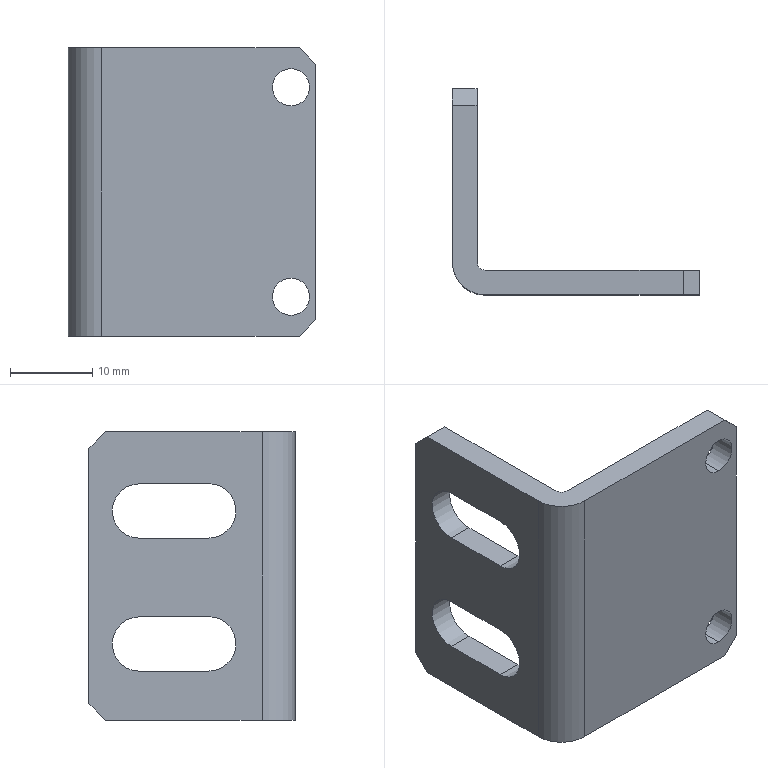Part | SolidWorks | features ICE 3, Chamfer 2, DelFace 2, HoleWzd 2, MoveFace 2, BaseBody 1 | 1 solid | 28 faces | box 30 x 25 x 35 mm | volume 4690 mm3 | plane 16 | cylinder 12 | commonest cylinder face diameters 6.6 x6 4.5 x4 2 x1 8 x1
STEP:
#1=CARTESIAN_POINT('',(-7.,3.,2.55));
#2=VERTEX_POINT('',#1);
#3=CARTESIAN_POINT('',(-7.,3.,7.05));
#4=VERTEX_POINT('',#3);
#5=CARTESIAN_POINT('',(-7.,3.,4.8));
#6=DIRECTION('',(0.,1.,0.));
#7=DIRECTION('',(0.,0.,1.));
#8=AXIS2_PLACEMENT_3D('',#5,#6,#7);
#9=CIRCLE('',#8,2.25);
#10=EDGE_CURVE('',#2,#4,#9,.T.);
#11=ORIENTED_EDGE('',*,*,#10,.T.);
#12=CARTESIAN_POINT('',(-7.,0.,7.05));
#13=VERTEX_POINT('',#12);
#14=CARTESIAN_POINT('',(-7.,0.,7.05));
#15=DIRECTION('',(0.,-1.,0.));
#16=VECTOR('',#15,1000.);
#17=LINE('',#14,#16);
#18=EDGE_CURVE('',#4,#13,#17,.T.);
#19=ORIENTED_EDGE('',*,*,#18,.T.);
#20=CARTESIAN_POINT('',(-7.,0.,2.55));
#21=VERTEX_POINT('',#20);
#22=CARTESIAN_POINT('',(-7.,0.,4.8));
#23=DIRECTION('',(0.,-1.,0.));
#24=DIRECTION('',(0.,0.,-1.));
#25=AXIS2_PLACEMENT_3D('',#22,#23,#24);
#26=CIRCLE('',#25,2.25);
#27=EDGE_CURVE('',#13,#21,#26,.T.);
#28=ORIENTED_EDGE('',*,*,#27,.T.);
#29=CARTESIAN_POINT('',(-7.,0.,2.55));
#30=DIRECTION('',(0.,-1.,0.));
#31=VECTOR('',#30,1000.);
#32=LINE('',#29,#31);
#33=EDGE_CURVE('',#2,#21,#32,.T.);
#34=ORIENTED_EDGE('',*,*,#33,.F.);
#35=EDGE_LOOP('',(#11,#19,#28,#34));
#36=FACE_OUTER_BOUND('',#35,.T.);
#37=CARTESIAN_POINT('',(-7.,0.,4.8));
#38=DIRECTION('',(0.,-1.,0.));
#39=DIRECTION('',(0.,0.,-1.));
#40=AXIS2_PLACEMENT_3D('',#37,#38,#39);
#41=CYLINDRICAL_SURFACE('',#40,2.25);
#42=ADVANCED_FACE('',(#36),#41,.F.);
#43=CARTESIAN_POINT('',(-7.,3.,27.95));
#44=VERTEX_POINT('',#43);
#45=CARTESIAN_POINT('',(-7.,3.,32.45));
#46=VERTEX_POINT('',#45);
#47=CARTESIAN_POINT('',(-7.,3.,30.2));
#48=DIRECTION('',(0.,1.,0.));
#49=DIRECTION('',(0.,0.,1.));
#50=AXIS2_PLACEMENT_3D('',#47,#48,#49);
#51=CIRCLE('',#50,2.25);
#52=EDGE_CURVE('',#44,#46,#51,.T.);
#53=ORIENTED_EDGE('',*,*,#52,.T.);
#54=CARTESIAN_POINT('',(-7.,0.,32.45));
#55=VERTEX_POINT('',#54);
#56=CARTESIAN_POINT('',(-7.,0.,32.45));
#57=DIRECTION('',(0.,-1.,0.));
#58=VECTOR('',#57,1000.);
#59=LINE('',#56,#58);
#60=EDGE_CURVE('',#46,#55,#59,.T.);
#61=ORIENTED_EDGE('',*,*,#60,.T.);
#62=CARTESIAN_POINT('',(-7.,0.,27.95));
#63=VERTEX_POINT('',#62);
#64=CARTESIAN_POINT('',(-7.,0.,30.2));
#65=DIRECTION('',(0.,-1.,0.));
#66=DIRECTION('',(0.,0.,-1.));
#67=AXIS2_PLACEMENT_3D('',#64,#65,#66);
#68=CIRCLE('',#67,2.25);
#69=EDGE_CURVE('',#55,#63,#68,.T.);
#70=ORIENTED_EDGE('',*,*,#69,.T.);
#71=CARTESIAN_POINT('',(-7.,0.,27.95));
#72=DIRECTION('',(0.,-1.,0.));
#73=VECTOR('',#72,1000.);
#74=LINE('',#71,#73);
#75=EDGE_CURVE('',#44,#63,#74,.T.);
#76=ORIENTED_EDGE('',*,*,#75,.F.);
#77=EDGE_LOOP('',(#53,#61,#70,#76));
#78=FACE_OUTER_BOUND('',#77,.T.);
#79=CARTESIAN_POINT('',(-7.,0.,30.2));
#80=DIRECTION('',(0.,-1.,0.));
#81=DIRECTION('',(0.,0.,-1.));
#82=AXIS2_PLACEMENT_3D('',#79,#80,#81);
#83=CYLINDRICAL_SURFACE('',#82,2.25);
#84=ADVANCED_FACE('',(#78),#83,.F.);
#85=CARTESIAN_POINT('',(-31.,10.466,12.573));
#86=VERTEX_POINT('',#85);
#87=CARTESIAN_POINT('',(-31.,10.476,12.573));
#88=VERTEX_POINT('',#87);
#89=CARTESIAN_POINT('',(-31.,10.466,9.273));
#90=DIRECTION('',(-1.,0.,0.));
#91=DIRECTION('',(0.,0.,1.));
#92=AXIS2_PLACEMENT_3D('',#89,#90,#91);
#93=CIRCLE('',#92,3.3);
#94=EDGE_CURVE('',#86,#88,#93,.T.);
#95=ORIENTED_EDGE('',*,*,#94,.F.);
#96=CARTESIAN_POINT('',(-34.,10.466,12.573));
#97=VERTEX_POINT('',#96);
#98=CARTESIAN_POINT('',(-34.,10.466,12.573));
#99=DIRECTION('',(-1.,0.,0.));
#100=VECTOR('',#99,1000.);
#101=LINE('',#98,#100);
#102=EDGE_CURVE('',#86,#97,#101,.T.);
#103=ORIENTED_EDGE('',*,*,#102,.T.);
#104=CARTESIAN_POINT('',(-34.,10.476,12.573));
#105=VERTEX_POINT('',#104);
#106=CARTESIAN_POINT('',(-34.,10.466,9.273));
#107=DIRECTION('',(-1.,0.,0.));
#108=DIRECTION('',(0.,0.,1.));
#109=AXIS2_PLACEMENT_3D('',#106,#107,#108);
#110=CIRCLE('',#109,3.3);
#111=EDGE_CURVE('',#97,#105,#110,.T.);
#112=ORIENTED_EDGE('',*,*,#111,.T.);
#113=CARTESIAN_POINT('',(-34.,10.476,12.573));
#114=DIRECTION('',(-1.,0.,0.));
#115=VECTOR('',#114,1000.);
#116=LINE('',#113,#115);
#117=EDGE_CURVE('',#88,#105,#116,.T.);
#118=ORIENTED_EDGE('',*,*,#117,.F.);
#119=EDGE_LOOP('',(#95,#103,#112,#118));
#120=FACE_OUTER_BOUND('',#119,.T.);
#121=CARTESIAN_POINT('',(-34.,10.466,9.273));
#122=DIRECTION('',(-1.,0.,0.));
#123=DIRECTION('',(0.,0.,1.));
#124=AXIS2_PLACEMENT_3D('',#121,#122,#123);
#125=CYLINDRICAL_SURFACE('',#124,3.3);
#126=ADVANCED_FACE('',(#120),#125,.F.);
#127=CARTESIAN_POINT('',(-31.,10.466,28.701));
#128=VERTEX_POINT('',#127);
#129=CARTESIAN_POINT('',(-31.,10.476,28.701));
#130=VERTEX_POINT('',#129);
#131=CARTESIAN_POINT('',(-31.,10.466,25.401));
#132=DIRECTION('',(-1.,0.,0.));
#133=DIRECTION('',(0.,0.,1.));
#134=AXIS2_PLACEMENT_3D('',#131,#132,#133);
#135=CIRCLE('',#134,3.3);
#136=EDGE_CURVE('',#128,#130,#135,.T.);
#137=ORIENTED_EDGE('',*,*,#136,.F.);
#138=CARTESIAN_POINT('',(-34.,10.466,28.701));
#139=VERTEX_POINT('',#138);
#140=CARTESIAN_POINT('',(-34.,10.466,28.701));
#141=DIRECTION('',(-1.,0.,0.));
#142=VECTOR('',#141,1000.);
#143=LINE('',#140,#142);
#144=EDGE_CURVE('',#128,#139,#143,.T.);
#145=ORIENTED_EDGE('',*,*,#144,.T.);
#146=CARTESIAN_POINT('',(-34.,10.476,28.701));
#147=VERTEX_POINT('',#146);
#148=CARTESIAN_POINT('',(-34.,10.466,25.401));
#149=DIRECTION('',(-1.,0.,0.));
#150=DIRECTION('',(0.,0.,1.));
#151=AXIS2_PLACEMENT_3D('',#148,#149,#150);
#152=CIRCLE('',#151,3.3);
#153=EDGE_CURVE('',#139,#147,#152,.T.);
#154=ORIENTED_EDGE('',*,*,#153,.T.);
#155=CARTESIAN_POINT('',(-34.,10.476,28.701));
#156=DIRECTION('',(-1.,0.,0.));
#157=VECTOR('',#156,1000.);
#158=LINE('',#155,#157);
#159=EDGE_CURVE('',#130,#147,#158,.T.);
#160=ORIENTED_EDGE('',*,*,#159,.F.);
#161=EDGE_LOOP('',(#137,#145,#154,#160));
#162=FACE_OUTER_BOUND('',#161,.T.);
#163=CARTESIAN_POINT('',(-34.,10.466,25.401));
#164=DIRECTION('',(-1.,0.,0.));
#165=DIRECTION('',(0.,0.,1.));
#166=AXIS2_PLACEMENT_3D('',#163,#164,#165);
#167=CYLINDRICAL_SURFACE('',#166,3.3);
#168=ADVANCED_FACE('',(#162),#167,.F.);
#169=CARTESIAN_POINT('',(-34.,18.876,28.677));
#170=VERTEX_POINT('',#169);
#171=CARTESIAN_POINT('',(-34.,18.876,28.677));
#172=DIRECTION('',(0.,-1.,0.002802));
#173=VECTOR('',#172,1000.);
#174=LINE('',#171,#173);
#175=EDGE_CURVE('',#170,#147,#174,.T.);
#176=ORIENTED_EDGE('',*,*,#175,.T.);
#177=ORIENTED_EDGE('',*,*,#153,.F.);
#178=CARTESIAN_POINT('',(-34.,10.457,22.101));
#179=VERTEX_POINT('',#178);
#180=CARTESIAN_POINT('',(-34.,10.466,25.401));
#181=DIRECTION('',(-1.,0.,0.));
#182=DIRECTION('',(0.,0.,1.));
#183=AXIS2_PLACEMENT_3D('',#180,#181,#182);
#184=CIRCLE('',#183,3.3);
#185=EDGE_CURVE('',#179,#139,#184,.T.);
#186=ORIENTED_EDGE('',*,*,#185,.F.);
#187=CARTESIAN_POINT('',(-34.,18.857,22.077));
#188=VERTEX_POINT('',#187);
#189=CARTESIAN_POINT('',(-34.,18.857,22.077));
#190=DIRECTION('',(0.,-1.,0.002802));
#191=VECTOR('',#190,1000.);
#192=LINE('',#189,#191);
#193=EDGE_CURVE('',#188,#179,#192,.T.);
#194=ORIENTED_EDGE('',*,*,#193,.F.);
#195=CARTESIAN_POINT('',(-34.,18.866,25.377));
#196=DIRECTION('',(-1.,0.,0.));
#197=DIRECTION('',(0.,0.,1.));
#198=AXIS2_PLACEMENT_3D('',#195,#196,#197);
#199=CIRCLE('',#198,3.3);
#200=EDGE_CURVE('',#170,#188,#199,.T.);
#201=ORIENTED_EDGE('',*,*,#200,.F.);
#202=EDGE_LOOP('',(#176,#177,#186,#194,#201));
#203=FACE_BOUND('',#202,.T.);
#204=CARTESIAN_POINT('',(-34.,4.,35.));
#205=VERTEX_POINT('',#204);
#206=CARTESIAN_POINT('',(-34.,23.,35.));
#207=VERTEX_POINT('',#206);
#208=CARTESIAN_POINT('',(-34.,0.,35.));
#209=DIRECTION('',(0.,1.,0.));
#210=VECTOR('',#209,1000.);
#211=LINE('',#208,#210);
#212=EDGE_CURVE('',#205,#207,#211,.T.);
#213=ORIENTED_EDGE('',*,*,#212,.T.);
#214=CARTESIAN_POINT('',(-34.,25.,33.));
#215=VERTEX_POINT('',#214);
#216=CARTESIAN_POINT('',(-34.,11.5,46.5));
#217=DIRECTION('',(0.,0.7071,-0.7071));
#218=VECTOR('',#217,1000.);
#219=LINE('',#216,#218);
#220=EDGE_CURVE('',#207,#215,#219,.T.);
#221=ORIENTED_EDGE('',*,*,#220,.T.);
#222=CARTESIAN_POINT('',(-34.,25.,2.));
#223=VERTEX_POINT('',#222);
#224=CARTESIAN_POINT('',(-34.,25.,35.));
#225=DIRECTION('',(0.,0.,-1.));
#226=VECTOR('',#225,1000.);
#227=LINE('',#224,#226);
#228=EDGE_CURVE('',#215,#223,#227,.T.);
#229=ORIENTED_EDGE('',*,*,#228,.T.);
#230=CARTESIAN_POINT('',(-34.,23.,0.));
#231=VERTEX_POINT('',#230);
#232=CARTESIAN_POINT('',(-34.,29.,6.));
#233=DIRECTION('',(0.,-0.7071,-0.7071));
#234=VECTOR('',#233,1000.);
#235=LINE('',#232,#234);
#236=EDGE_CURVE('',#223,#231,#235,.T.);
#237=ORIENTED_EDGE('',*,*,#236,.T.);
#238=CARTESIAN_POINT('',(-34.,4.,0.));
#239=VERTEX_POINT('',#238);
#240=CARTESIAN_POINT('',(-34.,0.,0.));
#241=DIRECTION('',(0.,1.,0.));
#242=VECTOR('',#241,1000.);
#243=LINE('',#240,#242);
#244=EDGE_CURVE('',#239,#231,#243,.T.);
#245=ORIENTED_EDGE('',*,*,#244,.F.);
#246=CARTESIAN_POINT('',(-34.,4.,35.));
#247=DIRECTION('',(0.,0.,-1.));
#248=VECTOR('',#247,1000.);
#249=LINE('',#246,#248);
#250=EDGE_CURVE('',#205,#239,#249,.T.);
#251=ORIENTED_EDGE('',*,*,#250,.F.);
#252=EDGE_LOOP('',(#213,#221,#229,#237,#245,#251));
#253=FACE_OUTER_BOUND('',#252,.T.);
#254=CARTESIAN_POINT('',(-34.,18.876,12.55));
#255=VERTEX_POINT('',#254);
#256=CARTESIAN_POINT('',(-34.,18.857,5.95));
#257=VERTEX_POINT('',#256);
#258=CARTESIAN_POINT('',(-34.,18.866,9.25));
#259=DIRECTION('',(-1.,0.,0.));
#260=DIRECTION('',(0.,0.,1.));
#261=AXIS2_PLACEMENT_3D('',#258,#259,#260);
#262=CIRCLE('',#261,3.3);
#263=EDGE_CURVE('',#255,#257,#262,.T.);
#264=ORIENTED_EDGE('',*,*,#263,.F.);
#265=CARTESIAN_POINT('',(-34.,18.876,12.55));
#266=DIRECTION('',(0.,-1.,0.002802));
#267=VECTOR('',#266,1000.);
#268=LINE('',#265,#267);
#269=EDGE_CURVE('',#255,#105,#268,.T.);
#270=ORIENTED_EDGE('',*,*,#269,.T.);
#271=ORIENTED_EDGE('',*,*,#111,.F.);
#272=CARTESIAN_POINT('',(-34.,10.457,5.973));
#273=VERTEX_POINT('',#272);
#274=CARTESIAN_POINT('',(-34.,10.466,9.273));
#275=DIRECTION('',(-1.,0.,0.));
#276=DIRECTION('',(0.,0.,1.));
#277=AXIS2_PLACEMENT_3D('',#274,#275,#276);
#278=CIRCLE('',#277,3.3);
#279=EDGE_CURVE('',#273,#97,#278,.T.);
#280=ORIENTED_EDGE('',*,*,#279,.F.);
#281=CARTESIAN_POINT('',(-34.,18.857,5.95));
#282=DIRECTION('',(0.,-1.,0.002802));
#283=VECTOR('',#282,1000.);
#284=LINE('',#281,#283);
#285=EDGE_CURVE('',#257,#273,#284,.T.);
#286=ORIENTED_EDGE('',*,*,#285,.F.);
#287=EDGE_LOOP('',(#264,#270,#271,#280,#286));
#288=FACE_BOUND('',#287,.T.);
#289=CARTESIAN_POINT('',(-34.,0.,35.));
#290=DIRECTION('',(-1.,0.,0.));
#291=DIRECTION('',(0.,0.,1.));
#292=AXIS2_PLACEMENT_3D('',#289,#290,#291);
#293=PLANE('',#292);
#294=ADVANCED_FACE('',(#203,#253,#288),#293,.T.);
#295=CARTESIAN_POINT('',(-30.,0.,35.));
#296=VERTEX_POINT('',#295);
#297=CARTESIAN_POINT('',(-6.,0.,35.));
#298=VERTEX_POINT('',#297);
#299=CARTESIAN_POINT('',(-30.,0.,35.));
#300=DIRECTION('',(1.,0.,0.));
#301=VECTOR('',#300,1000.);
#302=LINE('',#299,#301);
#303=EDGE_CURVE('',#296,#298,#302,.T.);
#304=ORIENTED_EDGE('',*,*,#303,.T.);
#305=CARTESIAN_POINT('',(-6.,3.,35.));
#306=VERTEX_POINT('',#305);
#307=CARTESIAN_POINT('',(-6.,3.,35.));
#308=DIRECTION('',(0.,1.,0.));
#309=VECTOR('',#308,1000.);
#310=LINE('',#307,#309);
#311=EDGE_CURVE('',#298,#306,#310,.T.);
#312=ORIENTED_EDGE('',*,*,#311,.T.);
#313=CARTESIAN_POINT('',(-30.,3.,35.));
#314=VERTEX_POINT('',#313);
#315=CARTESIAN_POINT('',(-30.,3.,35.));
#316=DIRECTION('',(1.,0.,0.));
#317=VECTOR('',#316,1000.);
#318=LINE('',#315,#317);
#319=EDGE_CURVE('',#314,#306,#318,.T.);
#320=ORIENTED_EDGE('',*,*,#319,.F.);
#321=CARTESIAN_POINT('',(-31.,4.,35.));
#322=VERTEX_POINT('',#321);
#323=CARTESIAN_POINT('',(-30.,4.,35.));
#324=DIRECTION('',(0.,0.,1.));
#325=DIRECTION('',(-1.,0.,0.));
#326=AXIS2_PLACEMENT_3D('',#323,#324,#325);
#327=CIRCLE('',#326,1.);
#328=EDGE_CURVE('',#322,#314,#327,.T.);
#329=ORIENTED_EDGE('',*,*,#328,.F.);
#330=CARTESIAN_POINT('',(-31.,23.,35.));
#331=VERTEX_POINT('',#330);
#332=CARTESIAN_POINT('',(-31.,0.,35.));
#333=DIRECTION('',(0.,1.,0.));
#334=VECTOR('',#333,1000.);
#335=LINE('',#332,#334);
#336=EDGE_CURVE('',#322,#331,#335,.T.);
#337=ORIENTED_EDGE('',*,*,#336,.T.);
#338=CARTESIAN_POINT('',(-34.,23.,35.));
#339=DIRECTION('',(-1.,0.,0.));
#340=VECTOR('',#339,1000.);
#341=LINE('',#338,#340);
#342=EDGE_CURVE('',#331,#207,#341,.T.);
#343=ORIENTED_EDGE('',*,*,#342,.T.);
#344=ORIENTED_EDGE('',*,*,#212,.F.);
#345=CARTESIAN_POINT('',(-30.,4.,35.));
#346=DIRECTION('',(0.,0.,1.));
#347=DIRECTION('',(-1.,0.,0.));
#348=AXIS2_PLACEMENT_3D('',#345,#346,#347);
#349=CIRCLE('',#348,4.);
#350=EDGE_CURVE('',#205,#296,#349,.T.);
#351=ORIENTED_EDGE('',*,*,#350,.T.);
#352=EDGE_LOOP('',(#304,#312,#320,#329,#337,#343,#344,#351));
#353=FACE_OUTER_BOUND('',#352,.T.);
#354=CARTESIAN_POINT('',(-3.,4.,35.));
#355=DIRECTION('',(0.,0.,1.));
#356=DIRECTION('',(1.,0.,0.));
#357=AXIS2_PLACEMENT_3D('',#354,#355,#356);
#358=PLANE('',#357);
#359=ADVANCED_FACE('',(#353),#358,.T.);
#360=ORIENTED_EDGE('',*,*,#10,.F.);
#361=CARTESIAN_POINT('',(-7.,3.,4.8));
#362=DIRECTION('',(0.,1.,0.));
#363=DIRECTION('',(0.,0.,1.));
#364=AXIS2_PLACEMENT_3D('',#361,#362,#363);
#365=CIRCLE('',#364,2.25);
#366=EDGE_CURVE('',#4,#2,#365,.T.);
#367=ORIENTED_EDGE('',*,*,#366,.F.);
#368=EDGE_LOOP('',(#360,#367));
#369=FACE_BOUND('',#368,.T.);
#370=ORIENTED_EDGE('',*,*,#52,.F.);
#371=CARTESIAN_POINT('',(-7.,3.,30.2));
#372=DIRECTION('',(0.,1.,0.));
#373=DIRECTION('',(0.,0.,1.));
#374=AXIS2_PLACEMENT_3D('',#371,#372,#373);
#375=CIRCLE('',#374,2.25);
#376=EDGE_CURVE('',#46,#44,#375,.T.);
#377=ORIENTED_EDGE('',*,*,#376,.F.);
#378=EDGE_LOOP('',(#370,#377));
#379=FACE_BOUND('',#378,.T.);
#380=ORIENTED_EDGE('',*,*,#319,.T.);
#381=CARTESIAN_POINT('',(-4.,3.,33.));
#382=VERTEX_POINT('',#381);
#383=CARTESIAN_POINT('',(-18.,3.,47.));
#384=DIRECTION('',(0.7071,0.,-0.7071));
#385=VECTOR('',#384,1000.);
#386=LINE('',#383,#385);
#387=EDGE_CURVE('',#306,#382,#386,.T.);
#388=ORIENTED_EDGE('',*,*,#387,.T.);
#389=CARTESIAN_POINT('',(-4.,3.,2.));
#390=VERTEX_POINT('',#389);
#391=CARTESIAN_POINT('',(-4.,3.,35.));
#392=DIRECTION('',(0.,0.,-1.));
#393=VECTOR('',#392,1000.);
#394=LINE('',#391,#393);
#395=EDGE_CURVE('',#382,#390,#394,.T.);
#396=ORIENTED_EDGE('',*,*,#395,.T.);
#397=CARTESIAN_POINT('',(-6.,3.,0.));
#398=VERTEX_POINT('',#397);
#399=CARTESIAN_POINT('',(-0.5,3.,5.5));
#400=DIRECTION('',(-0.7071,0.,-0.7071));
#401=VECTOR('',#400,1000.);
#402=LINE('',#399,#401);
#403=EDGE_CURVE('',#390,#398,#402,.T.);
#404=ORIENTED_EDGE('',*,*,#403,.T.);
#405=CARTESIAN_POINT('',(-30.,3.,0.));
#406=VERTEX_POINT('',#405);
#407=CARTESIAN_POINT('',(-30.,3.,0.));
#408=DIRECTION('',(1.,0.,0.));
#409=VECTOR('',#408,1000.);
#410=LINE('',#407,#409);
#411=EDGE_CURVE('',#406,#398,#410,.T.);
#412=ORIENTED_EDGE('',*,*,#411,.F.);
#413=CARTESIAN_POINT('',(-30.,3.,35.));
#414=DIRECTION('',(0.,0.,-1.));
#415=VECTOR('',#414,1000.);
#416=LINE('',#413,#415);
#417=EDGE_CURVE('',#314,#406,#416,.T.);
#418=ORIENTED_EDGE('',*,*,#417,.F.);
#419=EDGE_LOOP('',(#380,#388,#396,#404,#412,#418));
#420=FACE_OUTER_BOUND('',#419,.T.);
#421=CARTESIAN_POINT('',(-30.,3.,35.));
#422=DIRECTION('',(0.,1.,0.));
#423=DIRECTION('',(0.,0.,1.));
#424=AXIS2_PLACEMENT_3D('',#421,#422,#423);
#425=PLANE('',#424);
#426=ADVANCED_FACE('',(#369,#379,#420),#425,.T.);
#427=CARTESIAN_POINT('',(-7.,0.,4.8));
#428=DIRECTION('',(0.,-1.,0.));
#429=DIRECTION('',(0.,0.,-1.));
#430=AXIS2_PLACEMENT_3D('',#427,#428,#429);
#431=CIRCLE('',#430,2.25);
#432=EDGE_CURVE('',#21,#13,#431,.T.);
#433=ORIENTED_EDGE('',*,*,#432,.F.);
#434=ORIENTED_EDGE('',*,*,#27,.F.);
#435=EDGE_LOOP('',(#433,#434));
#436=FACE_BOUND('',#435,.T.);
#437=CARTESIAN_POINT('',(-7.,0.,30.2));
#438=DIRECTION('',(0.,-1.,0.));
#439=DIRECTION('',(0.,0.,-1.));
#440=AXIS2_PLACEMENT_3D('',#437,#438,#439);
#441=CIRCLE('',#440,2.25);
#442=EDGE_CURVE('',#63,#55,#441,.T.);
#443=ORIENTED_EDGE('',*,*,#442,.F.);
#444=ORIENTED_EDGE('',*,*,#69,.F.);
#445=EDGE_LOOP('',(#443,#444));
#446=FACE_BOUND('',#445,.T.);
#447=CARTESIAN_POINT('',(-4.,0.,33.));
#448=VERTEX_POINT('',#447);
#449=CARTESIAN_POINT('',(-4.,0.,2.));
#450=VERTEX_POINT('',#449);
#451=CARTESIAN_POINT('',(-4.,0.,35.));
#452=DIRECTION('',(0.,0.,-1.));
#453=VECTOR('',#452,1000.);
#454=LINE('',#451,#453);
#455=EDGE_CURVE('',#448,#450,#454,.T.);
#456=ORIENTED_EDGE('',*,*,#455,.F.);
#457=CARTESIAN_POINT('',(-6.,0.,35.));
#458=DIRECTION('',(-0.7071,0.,0.7071));
#459=VECTOR('',#458,1000.);
#460=LINE('',#457,#459);
#461=EDGE_CURVE('',#448,#298,#460,.T.);
#462=ORIENTED_EDGE('',*,*,#461,.T.);
#463=ORIENTED_EDGE('',*,*,#303,.F.);
#464=CARTESIAN_POINT('',(-30.,0.,0.));
#465=VERTEX_POINT('',#464);
#466=CARTESIAN_POINT('',(-30.,0.,35.));
#467=DIRECTION('',(0.,0.,-1.));
#468=VECTOR('',#467,1000.);
#469=LINE('',#466,#468);
#470=EDGE_CURVE('',#296,#465,#469,.T.);
#471=ORIENTED_EDGE('',*,*,#470,.T.);
#472=CARTESIAN_POINT('',(-6.,0.,0.));
#473=VERTEX_POINT('',#472);
#474=CARTESIAN_POINT('',(-30.,0.,0.));
#475=DIRECTION('',(1.,0.,0.));
#476=VECTOR('',#475,1000.);
#477=LINE('',#474,#476);
#478=EDGE_CURVE('',#465,#473,#477,.T.);
#479=ORIENTED_EDGE('',*,*,#478,.T.);
#480=CARTESIAN_POINT('',(-6.,0.,0.));
#481=DIRECTION('',(0.7071,0.,0.7071));
#482=VECTOR('',#481,1000.);
#483=LINE('',#480,#482);
#484=EDGE_CURVE('',#473,#450,#483,.T.);
#485=ORIENTED_EDGE('',*,*,#484,.T.);
#486=EDGE_LOOP('',(#456,#462,#463,#471,#479,#485));
#487=FACE_OUTER_BOUND('',#486,.T.);
#488=CARTESIAN_POINT('',(-30.,0.,35.));
#489=DIRECTION('',(0.,1.,0.));
#490=DIRECTION('',(0.,0.,1.));
#491=AXIS2_PLACEMENT_3D('',#488,#489,#490);
#492=PLANE('',#491);
#493=ADVANCED_FACE('',(#436,#446,#487),#492,.F.);
#494=ORIENTED_EDGE('',*,*,#411,.T.);
#495=CARTESIAN_POINT('',(-6.,4.,0.));
#496=DIRECTION('',(0.,-1.,0.));
#497=VECTOR('',#496,1000.);
#498=LINE('',#495,#497);
#499=EDGE_CURVE('',#398,#473,#498,.T.);
#500=ORIENTED_EDGE('',*,*,#499,.T.);
#501=ORIENTED_EDGE('',*,*,#478,.F.);
#502=CARTESIAN_POINT('',(-30.,4.,0.));
#503=DIRECTION('',(0.,0.,1.));
#504=DIRECTION('',(-1.,0.,0.));
#505=AXIS2_PLACEMENT_3D('',#502,#503,#504);
#506=CIRCLE('',#505,4.);
#507=EDGE_CURVE('',#239,#465,#506,.T.);
#508=ORIENTED_EDGE('',*,*,#507,.F.);
#509=ORIENTED_EDGE('',*,*,#244,.T.);
#510=CARTESIAN_POINT('',(-31.,23.,0.));
#511=VERTEX_POINT('',#510);
#512=CARTESIAN_POINT('',(-4.,23.,0.));
#513=DIRECTION('',(1.,0.,0.));
#514=VECTOR('',#513,1000.);
#515=LINE('',#512,#514);
#516=EDGE_CURVE('',#231,#511,#515,.T.);
#517=ORIENTED_EDGE('',*,*,#516,.T.);
#518=CARTESIAN_POINT('',(-31.,4.,0.));
#519=VERTEX_POINT('',#518);
#520=CARTESIAN_POINT('',(-31.,0.,0.));
#521=DIRECTION('',(0.,1.,0.));
#522=VECTOR('',#521,1000.);
#523=LINE('',#520,#522);
#524=EDGE_CURVE('',#519,#511,#523,.T.);
#525=ORIENTED_EDGE('',*,*,#524,.F.);
#526=CARTESIAN_POINT('',(-30.,4.,0.));
#527=DIRECTION('',(0.,0.,1.));
#528=DIRECTION('',(-1.,0.,0.));
#529=AXIS2_PLACEMENT_3D('',#526,#527,#528);
#530=CIRCLE('',#529,1.);
#531=EDGE_CURVE('',#519,#406,#530,.T.);
#532=ORIENTED_EDGE('',*,*,#531,.T.);
#533=EDGE_LOOP('',(#494,#500,#501,#508,#509,#517,#525,#532));
#534=FACE_OUTER_BOUND('',#533,.T.);
#535=CARTESIAN_POINT('',(-4.,4.,0.));
#536=DIRECTION('',(0.,0.,1.));
#537=DIRECTION('',(1.,0.,0.));
#538=AXIS2_PLACEMENT_3D('',#535,#536,#537);
#539=PLANE('',#538);
#540=ADVANCED_FACE('',(#534),#539,.F.);
#541=ORIENTED_EDGE('',*,*,#507,.T.);
#542=ORIENTED_EDGE('',*,*,#470,.F.);
#543=ORIENTED_EDGE('',*,*,#350,.F.);
#544=ORIENTED_EDGE('',*,*,#250,.T.);
#545=EDGE_LOOP('',(#541,#542,#543,#544));
#546=FACE_OUTER_BOUND('',#545,.T.);
#547=CARTESIAN_POINT('',(-30.,4.,35.));
#548=DIRECTION('',(0.,0.,-1.));
#549=DIRECTION('',(-1.,0.,0.));
#550=AXIS2_PLACEMENT_3D('',#547,#548,#549);
#551=CYLINDRICAL_SURFACE('',#550,4.);
#552=ADVANCED_FACE('',(#546),#551,.T.);
#553=ORIENTED_EDGE('',*,*,#531,.F.);
#554=CARTESIAN_POINT('',(-31.,4.,35.));
#555=DIRECTION('',(0.,0.,-1.));
#556=VECTOR('',#555,1000.);
#557=LINE('',#554,#556);
#558=EDGE_CURVE('',#322,#519,#557,.T.);
#559=ORIENTED_EDGE('',*,*,#558,.F.);
#560=ORIENTED_EDGE('',*,*,#328,.T.);
#561=ORIENTED_EDGE('',*,*,#417,.T.);
#562=EDGE_LOOP('',(#553,#559,#560,#561));
#563=FACE_OUTER_BOUND('',#562,.T.);
#564=CARTESIAN_POINT('',(-30.,4.,35.));
#565=DIRECTION('',(0.,0.,-1.));
#566=DIRECTION('',(-1.,0.,0.));
#567=AXIS2_PLACEMENT_3D('',#564,#565,#566);
#568=CYLINDRICAL_SURFACE('',#567,1.);
#569=ADVANCED_FACE('',(#563),#568,.F.);
#570=CARTESIAN_POINT('',(-31.,18.857,5.95));
#571=VERTEX_POINT('',#570);
#572=CARTESIAN_POINT('',(-31.,10.457,5.973));
#573=VERTEX_POINT('',#572);
#574=CARTESIAN_POINT('',(-31.,-0.08125,6.003));
#575=DIRECTION('',(0.,-1.,0.002802));
#576=VECTOR('',#575,1000.);
#577=LINE('',#574,#576);
#578=EDGE_CURVE('',#571,#573,#577,.T.);
#579=ORIENTED_EDGE('',*,*,#578,.T.);
#580=CARTESIAN_POINT('',(-31.,10.466,9.273));
#581=DIRECTION('',(-1.,0.,0.));
#582=DIRECTION('',(0.,0.,1.));
#583=AXIS2_PLACEMENT_3D('',#580,#581,#582);
#584=CIRCLE('',#583,3.3);
#585=EDGE_CURVE('',#573,#86,#584,.T.);
#586=ORIENTED_EDGE('',*,*,#585,.T.);
#587=ORIENTED_EDGE('',*,*,#94,.T.);
#588=CARTESIAN_POINT('',(-31.,18.876,12.55));
#589=VERTEX_POINT('',#588);
#590=CARTESIAN_POINT('',(-31.,-0.06275,12.603));
#591=DIRECTION('',(0.,1.,-0.002802));
#592=VECTOR('',#591,1000.);
#593=LINE('',#590,#592);
#594=EDGE_CURVE('',#88,#589,#593,.T.);
#595=ORIENTED_EDGE('',*,*,#594,.T.);
#596=CARTESIAN_POINT('',(-31.,18.866,9.25));
#597=DIRECTION('',(-1.,0.,0.));
#598=DIRECTION('',(0.,0.,1.));
#599=AXIS2_PLACEMENT_3D('',#596,#597,#598);
#600=CIRCLE('',#599,3.3);
#601=EDGE_CURVE('',#589,#571,#600,.T.);
#602=ORIENTED_EDGE('',*,*,#601,.T.);
#603=EDGE_LOOP('',(#579,#586,#587,#595,#602));
#604=FACE_BOUND('',#603,.T.);
#605=CARTESIAN_POINT('',(-31.,18.857,22.077));
#606=VERTEX_POINT('',#605);
#607=CARTESIAN_POINT('',(-31.,10.457,22.101));
#608=VERTEX_POINT('',#607);
#609=CARTESIAN_POINT('',(-31.,-0.03606,22.13));
#610=DIRECTION('',(0.,-1.,0.002802));
#611=VECTOR('',#610,1000.);
#612=LINE('',#609,#611);
#613=EDGE_CURVE('',#606,#608,#612,.T.);
#614=ORIENTED_EDGE('',*,*,#613,.T.);
#615=CARTESIAN_POINT('',(-31.,10.466,25.401));
#616=DIRECTION('',(-1.,0.,0.));
#617=DIRECTION('',(0.,0.,1.));
#618=AXIS2_PLACEMENT_3D('',#615,#616,#617);
#619=CIRCLE('',#618,3.3);
#620=EDGE_CURVE('',#608,#128,#619,.T.);
#621=ORIENTED_EDGE('',*,*,#620,.T.);
#622=ORIENTED_EDGE('',*,*,#136,.T.);
#623=CARTESIAN_POINT('',(-31.,18.876,28.677));
#624=VERTEX_POINT('',#623);
#625=CARTESIAN_POINT('',(-31.,-0.01757,28.73));
#626=DIRECTION('',(0.,1.,-0.002802));
#627=VECTOR('',#626,1000.);
#628=LINE('',#625,#627);
#629=EDGE_CURVE('',#130,#624,#628,.T.);
#630=ORIENTED_EDGE('',*,*,#629,.T.);
#631=CARTESIAN_POINT('',(-31.,18.866,25.377));
#632=DIRECTION('',(-1.,0.,0.));
#633=DIRECTION('',(0.,0.,1.));
#634=AXIS2_PLACEMENT_3D('',#631,#632,#633);
#635=CIRCLE('',#634,3.3);
#636=EDGE_CURVE('',#624,#606,#635,.T.);
#637=ORIENTED_EDGE('',*,*,#636,.T.);
#638=EDGE_LOOP('',(#614,#621,#622,#630,#637));
#639=FACE_BOUND('',#638,.T.);
#640=CARTESIAN_POINT('',(-31.,25.,33.));
#641=VERTEX_POINT('',#640);
#642=CARTESIAN_POINT('',(-31.,25.,2.));
#643=VERTEX_POINT('',#642);
#644=CARTESIAN_POINT('',(-31.,25.,35.));
#645=DIRECTION('',(0.,0.,-1.));
#646=VECTOR('',#645,1000.);
#647=LINE('',#644,#646);
#648=EDGE_CURVE('',#641,#643,#647,.T.);
#649=ORIENTED_EDGE('',*,*,#648,.F.);
#650=CARTESIAN_POINT('',(-31.,23.,35.));
#651=DIRECTION('',(0.,-0.7071,0.7071));
#652=VECTOR('',#651,1000.);
#653=LINE('',#650,#652);
#654=EDGE_CURVE('',#641,#331,#653,.T.);
#655=ORIENTED_EDGE('',*,*,#654,.T.);
#656=ORIENTED_EDGE('',*,*,#336,.F.);
#657=ORIENTED_EDGE('',*,*,#558,.T.);
#658=ORIENTED_EDGE('',*,*,#524,.T.);
#659=CARTESIAN_POINT('',(-31.,25.,2.));
#660=DIRECTION('',(0.,0.7071,0.7071));
#661=VECTOR('',#660,1000.);
#662=LINE('',#659,#661);
#663=EDGE_CURVE('',#511,#643,#662,.T.);
#664=ORIENTED_EDGE('',*,*,#663,.T.);
#665=EDGE_LOOP('',(#649,#655,#656,#657,#658,#664));
#666=FACE_OUTER_BOUND('',#665,.T.);
#667=CARTESIAN_POINT('',(-31.,0.,35.));
#668=DIRECTION('',(-1.,0.,0.));
#669=DIRECTION('',(0.,0.,1.));
#670=AXIS2_PLACEMENT_3D('',#667,#668,#669);
#671=PLANE('',#670);
#672=ADVANCED_FACE('',(#604,#639,#666),#671,.F.);
#673=ORIENTED_EDGE('',*,*,#228,.F.);
#674=CARTESIAN_POINT('',(-31.,25.,33.));
#675=DIRECTION('',(1.,0.,0.));
#676=VECTOR('',#675,1000.);
#677=LINE('',#674,#676);
#678=EDGE_CURVE('',#215,#641,#677,.T.);
#679=ORIENTED_EDGE('',*,*,#678,.T.);
#680=ORIENTED_EDGE('',*,*,#648,.T.);
#681=CARTESIAN_POINT('',(0.,25.,2.));
#682=DIRECTION('',(-1.,0.,0.));
#683=VECTOR('',#682,1000.);
#684=LINE('',#681,#683);
#685=EDGE_CURVE('',#643,#223,#684,.T.);
#686=ORIENTED_EDGE('',*,*,#685,.T.);
#687=EDGE_LOOP('',(#673,#679,#680,#686));
#688=FACE_OUTER_BOUND('',#687,.T.);
#689=CARTESIAN_POINT('',(0.,25.,35.));
#690=DIRECTION('',(0.,-1.,0.));
#691=DIRECTION('',(0.,0.,-1.));
#692=AXIS2_PLACEMENT_3D('',#689,#690,#691);
#693=PLANE('',#692);
#694=ADVANCED_FACE('',(#688),#693,.F.);
#695=ORIENTED_EDGE('',*,*,#144,.F.);
#696=ORIENTED_EDGE('',*,*,#620,.F.);
#697=CARTESIAN_POINT('',(-34.,10.457,22.101));
#698=DIRECTION('',(1.,0.,0.));
#699=VECTOR('',#698,1000.);
#700=LINE('',#697,#699);
#701=EDGE_CURVE('',#179,#608,#700,.T.);
#702=ORIENTED_EDGE('',*,*,#701,.F.);
#703=ORIENTED_EDGE('',*,*,#185,.T.);
#704=EDGE_LOOP('',(#695,#696,#702,#703));
#705=FACE_OUTER_BOUND('',#704,.T.);
#706=CARTESIAN_POINT('',(-34.,10.466,25.401));
#707=DIRECTION('',(-1.,0.,0.));
#708=DIRECTION('',(0.,0.,1.));
#709=AXIS2_PLACEMENT_3D('',#706,#707,#708);
#710=CYLINDRICAL_SURFACE('',#709,3.3);
#711=ADVANCED_FACE('',(#705),#710,.F.);
#712=CARTESIAN_POINT('',(-34.,18.857,22.077));
#713=DIRECTION('',(-1.,0.,0.));
#714=VECTOR('',#713,1000.);
#715=LINE('',#712,#714);
#716=EDGE_CURVE('',#606,#188,#715,.T.);
#717=ORIENTED_EDGE('',*,*,#716,.T.);
#718=ORIENTED_EDGE('',*,*,#193,.T.);
#719=ORIENTED_EDGE('',*,*,#701,.T.);
#720=ORIENTED_EDGE('',*,*,#613,.F.);
#721=EDGE_LOOP('',(#717,#718,#719,#720));
#722=FACE_OUTER_BOUND('',#721,.T.);
#723=CARTESIAN_POINT('',(-34.,18.857,22.077));
#724=DIRECTION('',(0.,-0.002802,-1.));
#725=DIRECTION('',(0.,1.,-0.002802));
#726=AXIS2_PLACEMENT_3D('',#723,#724,#725);
#727=PLANE('',#726);
#728=ADVANCED_FACE('',(#722),#727,.F.);
#729=ORIENTED_EDGE('',*,*,#159,.T.);
#730=ORIENTED_EDGE('',*,*,#175,.F.);
#731=CARTESIAN_POINT('',(-34.,18.876,28.677));
#732=DIRECTION('',(1.,0.,0.));
#733=VECTOR('',#732,1000.);
#734=LINE('',#731,#733);
#735=EDGE_CURVE('',#170,#624,#734,.T.);
#736=ORIENTED_EDGE('',*,*,#735,.T.);
#737=ORIENTED_EDGE('',*,*,#629,.F.);
#738=EDGE_LOOP('',(#729,#730,#736,#737));
#739=FACE_OUTER_BOUND('',#738,.T.);
#740=CARTESIAN_POINT('',(-34.,18.876,28.677));
#741=DIRECTION('',(0.,0.002802,1.));
#742=DIRECTION('',(0.,-1.,0.002802));
#743=AXIS2_PLACEMENT_3D('',#740,#741,#742);
#744=PLANE('',#743);
#745=ADVANCED_FACE('',(#739),#744,.F.);
#746=ORIENTED_EDGE('',*,*,#735,.F.);
#747=ORIENTED_EDGE('',*,*,#200,.T.);
#748=ORIENTED_EDGE('',*,*,#716,.F.);
#749=ORIENTED_EDGE('',*,*,#636,.F.);
#750=EDGE_LOOP('',(#746,#747,#748,#749));
#751=FACE_OUTER_BOUND('',#750,.T.);
#752=CARTESIAN_POINT('',(-34.,18.866,25.377));
#753=DIRECTION('',(-1.,0.,0.));
#754=DIRECTION('',(0.,0.,1.));
#755=AXIS2_PLACEMENT_3D('',#752,#753,#754);
#756=CYLINDRICAL_SURFACE('',#755,3.3);
#757=ADVANCED_FACE('',(#751),#756,.F.);
#758=CARTESIAN_POINT('',(-34.,18.857,5.95));
#759=DIRECTION('',(-1.,0.,0.));
#760=VECTOR('',#759,1000.);
#761=LINE('',#758,#760);
#762=EDGE_CURVE('',#571,#257,#761,.T.);
#763=ORIENTED_EDGE('',*,*,#762,.T.);
#764=ORIENTED_EDGE('',*,*,#285,.T.);
#765=CARTESIAN_POINT('',(-34.,10.457,5.973));
#766=DIRECTION('',(1.,0.,0.));
#767=VECTOR('',#766,1000.);
#768=LINE('',#765,#767);
#769=EDGE_CURVE('',#273,#573,#768,.T.);
#770=ORIENTED_EDGE('',*,*,#769,.T.);
#771=ORIENTED_EDGE('',*,*,#578,.F.);
#772=EDGE_LOOP('',(#763,#764,#770,#771));
#773=FACE_OUTER_BOUND('',#772,.T.);
#774=CARTESIAN_POINT('',(-34.,18.857,5.95));
#775=DIRECTION('',(0.,-0.002802,-1.));
#776=DIRECTION('',(0.,1.,-0.002802));
#777=AXIS2_PLACEMENT_3D('',#774,#775,#776);
#778=PLANE('',#777);
#779=ADVANCED_FACE('',(#773),#778,.F.);
#780=ORIENTED_EDGE('',*,*,#102,.F.);
#781=ORIENTED_EDGE('',*,*,#585,.F.);
#782=ORIENTED_EDGE('',*,*,#769,.F.);
#783=ORIENTED_EDGE('',*,*,#279,.T.);
#784=EDGE_LOOP('',(#780,#781,#782,#783));
#785=FACE_OUTER_BOUND('',#784,.T.);
#786=CARTESIAN_POINT('',(-34.,10.466,9.273));
#787=DIRECTION('',(-1.,0.,0.));
#788=DIRECTION('',(0.,0.,1.));
#789=AXIS2_PLACEMENT_3D('',#786,#787,#788);
#790=CYLINDRICAL_SURFACE('',#789,3.3);
#791=ADVANCED_FACE('',(#785),#790,.F.);
#792=ORIENTED_EDGE('',*,*,#117,.T.);
#793=ORIENTED_EDGE('',*,*,#269,.F.);
#794=CARTESIAN_POINT('',(-34.,18.876,12.55));
#795=DIRECTION('',(1.,0.,0.));
#796=VECTOR('',#795,1000.);
#797=LINE('',#794,#796);
#798=EDGE_CURVE('',#255,#589,#797,.T.);
#799=ORIENTED_EDGE('',*,*,#798,.T.);
#800=ORIENTED_EDGE('',*,*,#594,.F.);
#801=EDGE_LOOP('',(#792,#793,#799,#800));
#802=FACE_OUTER_BOUND('',#801,.T.);
#803=CARTESIAN_POINT('',(-34.,18.876,12.55));
#804=DIRECTION('',(0.,0.002802,1.));
#805=DIRECTION('',(0.,-1.,0.002802));
#806=AXIS2_PLACEMENT_3D('',#803,#804,#805);
#807=PLANE('',#806);
#808=ADVANCED_FACE('',(#802),#807,.F.);
#809=ORIENTED_EDGE('',*,*,#798,.F.);
#810=ORIENTED_EDGE('',*,*,#263,.T.);
#811=ORIENTED_EDGE('',*,*,#762,.F.);
#812=ORIENTED_EDGE('',*,*,#601,.F.);
#813=EDGE_LOOP('',(#809,#810,#811,#812));
#814=FACE_OUTER_BOUND('',#813,.T.);
#815=CARTESIAN_POINT('',(-34.,18.866,9.25));
#816=DIRECTION('',(-1.,0.,0.));
#817=DIRECTION('',(0.,0.,1.));
#818=AXIS2_PLACEMENT_3D('',#815,#816,#817);
#819=CYLINDRICAL_SURFACE('',#818,3.3);
#820=ADVANCED_FACE('',(#814),#819,.F.);
#821=ORIENTED_EDGE('',*,*,#654,.F.);
#822=ORIENTED_EDGE('',*,*,#678,.F.);
#823=ORIENTED_EDGE('',*,*,#220,.F.);
#824=ORIENTED_EDGE('',*,*,#342,.F.);
#825=EDGE_LOOP('',(#821,#822,#823,#824));
#826=FACE_OUTER_BOUND('',#825,.T.);
#827=CARTESIAN_POINT('',(-3.,23.,35.));
#828=DIRECTION('',(0.,0.7071,0.7071));
#829=DIRECTION('',(1.,0.,0.));
#830=AXIS2_PLACEMENT_3D('',#827,#828,#829);
#831=PLANE('',#830);
#832=ADVANCED_FACE('',(#826),#831,.T.);
#833=ORIENTED_EDGE('',*,*,#663,.F.);
#834=ORIENTED_EDGE('',*,*,#516,.F.);
#835=ORIENTED_EDGE('',*,*,#236,.F.);
#836=ORIENTED_EDGE('',*,*,#685,.F.);
#837=EDGE_LOOP('',(#833,#834,#835,#836));
#838=FACE_OUTER_BOUND('',#837,.T.);
#839=CARTESIAN_POINT('',(0.,25.,2.));
#840=DIRECTION('',(0.,-0.7071,0.7071));
#841=DIRECTION('',(-1.,0.,0.));
#842=AXIS2_PLACEMENT_3D('',#839,#840,#841);
#843=PLANE('',#842);
#844=ADVANCED_FACE('',(#838),#843,.F.);
#845=ORIENTED_EDGE('',*,*,#395,.F.);
#846=CARTESIAN_POINT('',(-4.,0.,33.));
#847=DIRECTION('',(0.,-1.,0.));
#848=VECTOR('',#847,1000.);
#849=LINE('',#846,#848);
#850=EDGE_CURVE('',#382,#448,#849,.T.);
#851=ORIENTED_EDGE('',*,*,#850,.T.);
#852=ORIENTED_EDGE('',*,*,#455,.T.);
#853=CARTESIAN_POINT('',(-4.,-28.,2.));
#854=DIRECTION('',(0.,1.,0.));
#855=VECTOR('',#854,1000.);
#856=LINE('',#853,#855);
#857=EDGE_CURVE('',#450,#390,#856,.T.);
#858=ORIENTED_EDGE('',*,*,#857,.T.);
#859=EDGE_LOOP('',(#845,#851,#852,#858));
#860=FACE_OUTER_BOUND('',#859,.T.);
#861=CARTESIAN_POINT('',(-4.,-28.,35.));
#862=DIRECTION('',(-1.,0.,0.));
#863=DIRECTION('',(0.,0.,1.));
#864=AXIS2_PLACEMENT_3D('',#861,#862,#863);
#865=PLANE('',#864);
#866=ADVANCED_FACE('',(#860),#865,.F.);
#867=ORIENTED_EDGE('',*,*,#461,.F.);
#868=ORIENTED_EDGE('',*,*,#850,.F.);
#869=ORIENTED_EDGE('',*,*,#387,.F.);
#870=ORIENTED_EDGE('',*,*,#311,.F.);
#871=EDGE_LOOP('',(#867,#868,#869,#870));
#872=FACE_OUTER_BOUND('',#871,.T.);
#873=CARTESIAN_POINT('',(-6.,4.,35.));
#874=DIRECTION('',(0.7071,0.,0.7071));
#875=DIRECTION('',(0.,-1.,0.));
#876=AXIS2_PLACEMENT_3D('',#873,#874,#875);
#877=PLANE('',#876);
#878=ADVANCED_FACE('',(#872),#877,.T.);
#879=ORIENTED_EDGE('',*,*,#403,.F.);
#880=ORIENTED_EDGE('',*,*,#857,.F.);
#881=ORIENTED_EDGE('',*,*,#484,.F.);
#882=ORIENTED_EDGE('',*,*,#499,.F.);
#883=EDGE_LOOP('',(#879,#880,#881,#882));
#884=FACE_OUTER_BOUND('',#883,.T.);
#885=CARTESIAN_POINT('',(-6.,4.,0.));
#886=DIRECTION('',(-0.7071,0.,0.7071));
#887=DIRECTION('',(0.,-1.,0.));
#888=AXIS2_PLACEMENT_3D('',#885,#886,#887);
#889=PLANE('',#888);
#890=ADVANCED_FACE('',(#884),#889,.F.);
#891=ORIENTED_EDGE('',*,*,#60,.F.);
#892=ORIENTED_EDGE('',*,*,#376,.T.);
#893=ORIENTED_EDGE('',*,*,#75,.T.);
#894=ORIENTED_EDGE('',*,*,#442,.T.);
#895=EDGE_LOOP('',(#891,#892,#893,#894));
#896=FACE_OUTER_BOUND('',#895,.T.);
#897=CARTESIAN_POINT('',(-7.,0.,30.2));
#898=DIRECTION('',(0.,-1.,0.));
#899=DIRECTION('',(0.,0.,-1.));
#900=AXIS2_PLACEMENT_3D('',#897,#898,#899);
#901=CYLINDRICAL_SURFACE('',#900,2.25);
#902=ADVANCED_FACE('',(#896),#901,.F.);
#903=ORIENTED_EDGE('',*,*,#18,.F.);
#904=ORIENTED_EDGE('',*,*,#366,.T.);
#905=ORIENTED_EDGE('',*,*,#33,.T.);
#906=ORIENTED_EDGE('',*,*,#432,.T.);
#907=EDGE_LOOP('',(#903,#904,#905,#906));
#908=FACE_OUTER_BOUND('',#907,.T.);
#909=CARTESIAN_POINT('',(-7.,0.,4.8));
#910=DIRECTION('',(0.,-1.,0.));
#911=DIRECTION('',(0.,0.,-1.));
#912=AXIS2_PLACEMENT_3D('',#909,#910,#911);
#913=CYLINDRICAL_SURFACE('',#912,2.25);
#914=ADVANCED_FACE('',(#908),#913,.F.);
#915=CLOSED_SHELL('',(#42,#84,#126,#168,#294,#359,#426,#493,#540,#552,#569,#672,#694,#711,#728,#745,#757,#779,#791,#808,#820,#832,#844,#866,#878,#890,#902,#914));
#916=MANIFOLD_SOLID_BREP('',#915);
#917=CARTESIAN_POINT('',(0.,0.,0.));
#918=DIRECTION('',(0.,0.,1.));
#919=DIRECTION('',(1.,0.,0.));
#920=AXIS2_PLACEMENT_3D('',#917,#918,#919);
#921=(LENGTH_UNIT()NAMED_UNIT(*)SI_UNIT(.MILLI.,.METRE.));
#922=UNCERTAINTY_MEASURE_WITH_UNIT(LENGTH_MEASURE(0.00001),#921,'','');
#923=(NAMED_UNIT(*)PLANE_ANGLE_UNIT()SI_UNIT($,.RADIAN.));
#924=(NAMED_UNIT(*)SI_UNIT($,.STERADIAN.)SOLID_ANGLE_UNIT());
#925=(GEOMETRIC_REPRESENTATION_CONTEXT(3)GLOBAL_UNCERTAINTY_ASSIGNED_CONTEXT((#922))GLOBAL_UNIT_ASSIGNED_CONTEXT((#921,#923,#924))REPRESENTATION_CONTEXT('',''));
#926=ADVANCED_BREP_SHAPE_REPRESENTATION('',(#916,#920),#925);